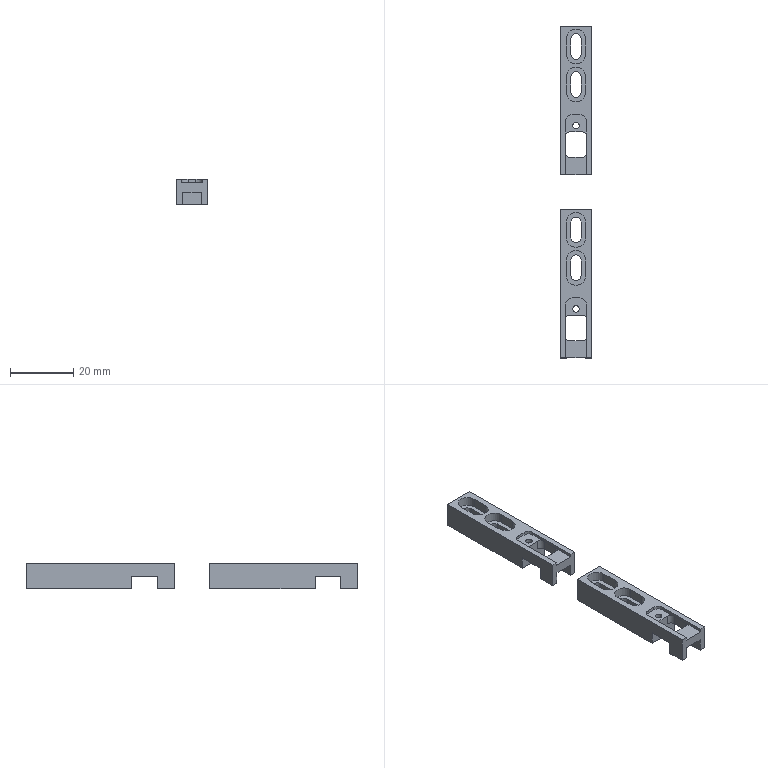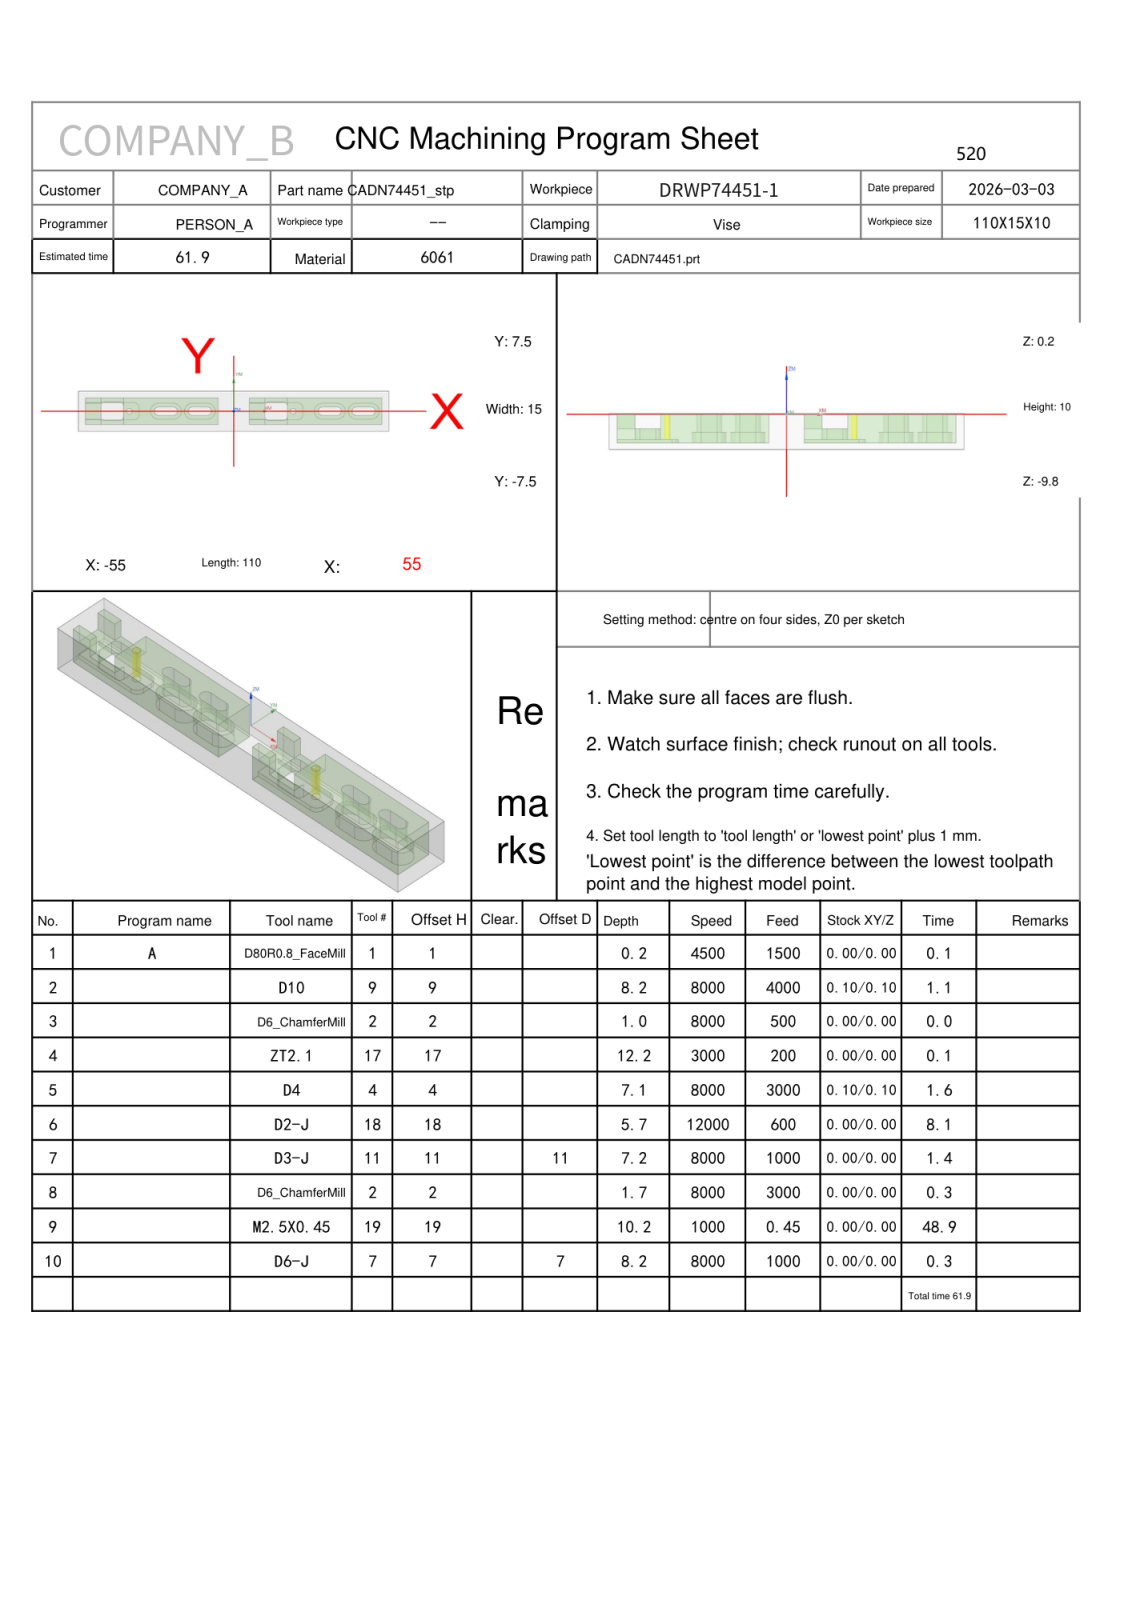NC program | NX | posted by the shop | part box 10 x 105 x 8 mm
Lines 1 to 2024 of 4761:
%
O0001
(Machine time: 108.11 MIN)
(===Total Tool:9===)
(T1=D80R0.8 FaceMill D=80.  R=0.8  D-  H01 Z=0.    )
(T9=D10     D=10.  R=0.   D-  H09 Z=-8.   )
(T2=D6_ChamferMill   D=6.   R=0.   D-  H02 Z=-1.5  )
(T17=ZT2.1  D=2.1  DR_a=118 D-  H17 Z=-12.  )
(T4=D4      D=4.   R=0.   D-  H04 Z=-6.9  )
(T18=D2-J   D=2.   R=0.   D18 H18 Z=-5.5  )
(T11=D3-J   D=3.   R=0.   D11 H11 Z=-7.   )
(T19=M2.5X0.45 D=2.05 DR_a=180 D-  H19 Z=-10.  )
(T7=D6-J    D=6.   R=0.   D7  H07 Z=-8.   )
G80 G90 G17 G49 G40
G91 G28 Z0
M01
N1 T01 M06
(D80R0.8 FaceMill  D=80. R=0.8 H=01 ce=0.00 di=0.00)
G00 G90 G54 X-97.5 Y0.0 M03 S4500
G43 H01 Z50.
M08
Z2.
G01 Z0.0 F1500.
X-92.5
X92.5
X97.5
Z2.
G00 Z50.
G91 G28 Z0.0
M05
M09
G91 G28 Z0.0
M01
N2 T09 M06
(D10  D=10. R=0. H=09 ce=0.10 di=0.10)
G00 G90 G54 X57.481 Y6.032 M03 S8000
G43 H09 Z50.
M08
Z1.
G01 X57.6 Y5.554 Z.974 F4000.
Y-5.554 Z.392
X57.266 Y-6.898 Z.319
X56.584 Y-8.104 Z.247
X55.604 Y-9.084 Z.174
X54.398 Y-9.766 Z.102
X53.054 Y-10.1 Z.029
X52.5 Z0.0
X5.5 Z-.184
G02 X.4 Y-5. Z-.215 I0.0 J5.1
G01 Y5. Z-.254
G02 X5.5 Y10.1 Z-.286 I5.1 J0.0
G01 X52.5 Z-.47
G02 X57.6 Y5. Z-.501 I0.0 J-5.1
G01 Y-5. Z-.54
G02 X52.5 Y-10.1 Z-.571 I-5.1 J0.0
G01 X5.5 Z-.755
G02 X.4 Y-5. Z-.787 I0.0 J5.1
G01 Y5. Z-.826
G02 X5.5 Y10.1 Z-.857 I5.1 J0.0
G01 X52.5 Z-1.041
G02 X57.6 Y5. Z-1.072 I0.0 J-5.1
G01 Y-5. Z-1.112
G02 X52.5 Y-10.1 Z-1.143 I-5.1 J0.0
G01 X5.5 Z-1.327
G02 X.4 Y-5. Z-1.358 I0.0 J5.1
G01 Y5. Z-1.397
G02 X5.5 Y10.1 Z-1.429 I5.1 J0.0
G01 X52.5 Z-1.612
G02 X57.6 Y5. Z-1.644 I0.0 J-5.1
G01 Y-5. Z-1.683
G02 X52.5 Y-10.1 Z-1.714 I-5.1 J0.0
G01 X5.5 Z-1.898
G02 X.4 Y-5. Z-1.93 I0.0 J5.1
G01 Y5. Z-1.969
G02 X5.5 Y10.1 Z-2. I5.1 J0.0
G01 X52.5 Z-2.184
G02 X57.6 Y5. Z-2.215 I0.0 J-5.1
G01 Y-5. Z-2.254
G02 X52.5 Y-10.1 Z-2.286 I-5.1 J0.0
G01 X5.5 Z-2.47
G02 X.4 Y-5. Z-2.501 I0.0 J5.1
G01 Y5. Z-2.54
G02 X5.5 Y10.1 Z-2.571 I5.1 J0.0
G01 X52.5 Z-2.755
G02 X57.6 Y5. Z-2.787 I0.0 J-5.1
G01 Y-5. Z-2.826
G02 X52.5 Y-10.1 Z-2.857 I-5.1 J0.0
G01 X5.5 Z-3.041
G02 X.4 Y-5. Z-3.072 I0.0 J5.1
G01 Y5. Z-3.112
G02 X5.5 Y10.1 Z-3.143 I5.1 J0.0
G01 X52.5 Z-3.327
G02 X57.6 Y5. Z-3.358 I0.0 J-5.1
G01 Y-5. Z-3.397
G02 X52.5 Y-10.1 Z-3.429 I-5.1 J0.0
G01 X5.5 Z-3.612
G02 X.4 Y-5. Z-3.644 I0.0 J5.1
G01 Y5. Z-3.683
G02 X5.5 Y10.1 Z-3.714 I5.1 J0.0
G01 X52.5 Z-3.898
G02 X57.6 Y5. Z-3.93 I0.0 J-5.1
G01 Y-5. Z-3.969
G02 X52.5 Y-10.1 Z-4. I-5.1 J0.0
G01 X5.5 Z-4.184
G02 X.4 Y-5. Z-4.215 I0.0 J5.1
G01 Y5. Z-4.254
G02 X5.5 Y10.1 Z-4.286 I5.1 J0.0
G01 X52.5 Z-4.47
G02 X57.6 Y5. Z-4.501 I0.0 J-5.1
G01 Y-5. Z-4.54
G02 X52.5 Y-10.1 Z-4.571 I-5.1 J0.0
G01 X5.5 Z-4.755
G02 X.4 Y-5. Z-4.787 I0.0 J5.1
G01 Y5. Z-4.826
G02 X5.5 Y10.1 Z-4.857 I5.1 J0.0
G01 X52.5 Z-5.041
G02 X57.6 Y5. Z-5.072 I0.0 J-5.1
G01 Y-5. Z-5.112
G02 X52.5 Y-10.1 Z-5.143 I-5.1 J0.0
G01 X5.5 Z-5.327
G02 X.4 Y-5. Z-5.358 I0.0 J5.1
G01 Y5. Z-5.397
G02 X5.5 Y10.1 Z-5.429 I5.1 J0.0
G01 X52.5 Z-5.612
G02 X57.6 Y5. Z-5.644 I0.0 J-5.1
G01 Y-5. Z-5.683
G02 X52.5 Y-10.1 Z-5.714 I-5.1 J0.0
G01 X5.5 Z-5.898
G02 X.4 Y-5. Z-5.93 I0.0 J5.1
G01 Y5. Z-5.969
G02 X5.5 Y10.1 Z-6. I5.1 J0.0
G01 X52.5 Z-6.184
G02 X57.6 Y5. Z-6.215 I0.0 J-5.1
G01 Y-5. Z-6.254
G02 X52.5 Y-10.1 Z-6.286 I-5.1 J0.0
G01 X5.5 Z-6.47
G02 X.4 Y-5. Z-6.501 I0.0 J5.1
G01 Y5. Z-6.54
G02 X5.5 Y10.1 Z-6.571 I5.1 J0.0
G01 X52.5 Z-6.755
G02 X57.6 Y5. Z-6.787 I0.0 J-5.1
G01 Y-5. Z-6.826
G02 X52.5 Y-10.1 Z-6.857 I-5.1 J0.0
G01 X5.5 Z-7.041
G02 X.4 Y-5. Z-7.072 I0.0 J5.1
G01 Y5. Z-7.112
G02 X5.5 Y10.1 Z-7.143 I5.1 J0.0
G01 X52.5 Z-7.327
G02 X57.6 Y5. Z-7.358 I0.0 J-5.1
G01 Y-5. Z-7.397
G02 X52.5 Y-10.1 Z-7.429 I-5.1 J0.0
G01 X5.5 Z-7.612
G02 X.4 Y-5. Z-7.644 I0.0 J5.1
G01 Y5. Z-7.683
G02 X5.5 Y10.1 Z-7.714 I5.1 J0.0
G01 X52.5 Z-7.898
G02 X57.6 Y5. Z-7.93 I0.0 J-5.1
G01 Y-5. Z-7.969
G02 X52.5 Y-10.1 Z-8. I-5.1 J0.0
G01 X5.5
G02 X.4 Y-5. I0.0 J5.1
G01 Y5.
G02 X5.5 Y10.1 I5.1 J0.0
G01 X52.5
G02 X57.6 Y5. I0.0 J-5.1
G01 Y-5.
G02 X52.5 Y-10.1 I-5.1 J0.0
G01 X52.1
Z-7.
G00 Z50.
X-48.081 Y10.1
Z1.
G01 X-29. Z0.0
X-5.5 Z-.092
G02 X-.4 Y5. Z-.123 I0.0 J-5.1
G01 Y-5. Z-.162
G02 X-5.5 Y-10.1 Z-.194 I-5.1 J0.0
G01 X-52.5 Z-.378
G02 X-57.6 Y-5. Z-.409 I0.0 J5.1
G01 Y5. Z-.448
G02 X-52.5 Y10.1 Z-.479 I5.1 J0.0
G01 X-5.5 Z-.663
G02 X-.4 Y5. Z-.695 I0.0 J-5.1
G01 Y-5. Z-.734
G02 X-5.5 Y-10.1 Z-.765 I-5.1 J0.0
G01 X-52.5 Z-.949
G02 X-57.6 Y-5. Z-.98 I0.0 J5.1
G01 Y5. Z-1.02
G02 X-52.5 Y10.1 Z-1.051 I5.1 J0.0
G01 X-5.5 Z-1.235
G02 X-.4 Y5. Z-1.266 I0.0 J-5.1
G01 Y-5. Z-1.305
G02 X-5.5 Y-10.1 Z-1.337 I-5.1 J0.0
G01 X-52.5 Z-1.521
G02 X-57.6 Y-5. Z-1.552 I0.0 J5.1
G01 Y5. Z-1.591
G02 X-52.5 Y10.1 Z-1.622 I5.1 J0.0
G01 X-5.5 Z-1.806
G02 X-.4 Y5. Z-1.838 I0.0 J-5.1
G01 Y-5. Z-1.877
G02 X-5.5 Y-10.1 Z-1.908 I-5.1 J0.0
G01 X-52.5 Z-2.092
G02 X-57.6 Y-5. Z-2.123 I0.0 J5.1
G01 Y5. Z-2.162
G02 X-52.5 Y10.1 Z-2.194 I5.1 J0.0
G01 X-5.5 Z-2.378
G02 X-.4 Y5. Z-2.409 I0.0 J-5.1
G01 Y-5. Z-2.448
G02 X-5.5 Y-10.1 Z-2.479 I-5.1 J0.0
G01 X-52.5 Z-2.663
G02 X-57.6 Y-5. Z-2.695 I0.0 J5.1
G01 Y5. Z-2.734
G02 X-52.5 Y10.1 Z-2.765 I5.1 J0.0
G01 X-5.5 Z-2.949
G02 X-.4 Y5. Z-2.98 I0.0 J-5.1
G01 Y-5. Z-3.02
G02 X-5.5 Y-10.1 Z-3.051 I-5.1 J0.0
G01 X-52.5 Z-3.235
G02 X-57.6 Y-5. Z-3.266 I0.0 J5.1
G01 Y5. Z-3.305
G02 X-52.5 Y10.1 Z-3.337 I5.1 J0.0
G01 X-5.5 Z-3.521
G02 X-.4 Y5. Z-3.552 I0.0 J-5.1
G01 Y-5. Z-3.591
G02 X-5.5 Y-10.1 Z-3.622 I-5.1 J0.0
G01 X-52.5 Z-3.806
G02 X-57.6 Y-5. Z-3.838 I0.0 J5.1
G01 Y5. Z-3.877
G02 X-52.5 Y10.1 Z-3.908 I5.1 J0.0
G01 X-5.5 Z-4.092
G02 X-.4 Y5. Z-4.123 I0.0 J-5.1
G01 Y-5. Z-4.162
G02 X-5.5 Y-10.1 Z-4.194 I-5.1 J0.0
G01 X-52.5 Z-4.378
G02 X-57.6 Y-5. Z-4.409 I0.0 J5.1
G01 Y5. Z-4.448
G02 X-52.5 Y10.1 Z-4.479 I5.1 J0.0
G01 X-5.5 Z-4.663
G02 X-.4 Y5. Z-4.695 I0.0 J-5.1
G01 Y-5. Z-4.734
G02 X-5.5 Y-10.1 Z-4.765 I-5.1 J0.0
G01 X-52.5 Z-4.949
G02 X-57.6 Y-5. Z-4.98 I0.0 J5.1
G01 Y5. Z-5.02
G02 X-52.5 Y10.1 Z-5.051 I5.1 J0.0
G01 X-5.5 Z-5.235
G02 X-.4 Y5. Z-5.266 I0.0 J-5.1
G01 Y-5. Z-5.305
G02 X-5.5 Y-10.1 Z-5.337 I-5.1 J0.0
G01 X-52.5 Z-5.521
G02 X-57.6 Y-5. Z-5.552 I0.0 J5.1
G01 Y5. Z-5.591
G02 X-52.5 Y10.1 Z-5.622 I5.1 J0.0
G01 X-5.5 Z-5.806
G02 X-.4 Y5. Z-5.838 I0.0 J-5.1
G01 Y-5. Z-5.877
G02 X-5.5 Y-10.1 Z-5.908 I-5.1 J0.0
G01 X-52.5 Z-6.092
G02 X-57.6 Y-5. Z-6.123 I0.0 J5.1
G01 Y5. Z-6.162
G02 X-52.5 Y10.1 Z-6.194 I5.1 J0.0
G01 X-5.5 Z-6.378
G02 X-.4 Y5. Z-6.409 I0.0 J-5.1
G01 Y-5. Z-6.448
G02 X-5.5 Y-10.1 Z-6.479 I-5.1 J0.0
G01 X-52.5 Z-6.663
G02 X-57.6 Y-5. Z-6.695 I0.0 J5.1
G01 Y5. Z-6.734
G02 X-52.5 Y10.1 Z-6.765 I5.1 J0.0
G01 X-5.5 Z-6.949
G02 X-.4 Y5. Z-6.98 I0.0 J-5.1
G01 Y-5. Z-7.02
G02 X-5.5 Y-10.1 Z-7.051 I-5.1 J0.0
G01 X-52.5 Z-7.235
G02 X-57.6 Y-5. Z-7.266 I0.0 J5.1
G01 Y5. Z-7.305
G02 X-52.5 Y10.1 Z-7.337 I5.1 J0.0
G01 X-5.5 Z-7.521
G02 X-.4 Y5. Z-7.552 I0.0 J-5.1
G01 Y-5. Z-7.591
G02 X-5.5 Y-10.1 Z-7.622 I-5.1 J0.0
G01 X-52.5 Z-7.806
G02 X-57.6 Y-5. Z-7.838 I0.0 J5.1
G01 Y5. Z-7.877
G02 X-52.5 Y10.1 Z-7.908 I5.1 J0.0
G01 X-29. Z-8.
X-5.5
G02 X-.4 Y5. I0.0 J-5.1
G01 Y-5.
G02 X-5.5 Y-10.1 I-5.1 J0.0
G01 X-52.5
G02 X-57.6 Y-5. I0.0 J5.1
G01 Y5.
G02 X-52.5 Y10.1 I5.1 J0.0
G01 X-29.
X-28.6
Z-7.
G00 Z50.
G91 G28 Z0.0
M05
M09
G91 G28 Z0.0
M01
N3 T02 M06
(D6_ChamferMill  D=6. R=0. H=02 ce=0.00 di=0.10)
G00 G90 G54 X21. Y0.0 M03 S8000
G43 H02 Z50.
M08
G98 G81 X21. Y0.0 Z-.8 R1. F500.
X-37.
G80
G00 Z50.
G91 G28 Z0.0
M05
M09
G91 G28 Z0.0
M01
N4 T17 M06
(ZT2.1 D=2.1 DR_a=118 H=17)
G00 G90 G54 X21. Y0.0 M03 S3000
G43 H17 Z50.
M08
G98 G83 X21. Y0.0 Z-12. R1. F200. Q2.
X-37.
G80
G00 Z50.
G91 G28 Z0.0
M05
M09
G91 G28 Z0.0
M01
N5 T04 M06
(D4  D=4. R=0. H=04 ce=0.10 di=0.10)
G00 G90 G54 X13.819 Y-1.4 M03 S8000
G43 H04 Z50.
M08
Z1.
G01 X16.9 Z.839 F2000.
Y1.4 Z.692
X13.1 Z.493
Y-1.4 Z.346
X16.9 Z.147
Y1.4 Z0.0
X13.1 Z-.083
Y-1.4 Z-.144
X16.9 Z-.227
Y1.4 Z-.288
X13.1 Z-.37
Y-1.4 Z-.431
X16.9 Z-.514
Y1.4 Z-.575
X13.1 Z-.658
Y-1.4 Z-.719
X16.9 Z-.802
Y1.4 Z-.863
X13.1 Z-.945
Y-1.4 Z-1.006
X16.9 Z-1.089
Y1.4 Z-1.15
X13.1 Z-1.233
Y-1.4 Z-1.294
X16.9 Z-1.377
Y1.4 Z-1.438
X13.1 Z-1.52
Y-1.4 Z-1.581
X16.9 Z-1.664
Y1.4 Z-1.725
X13.1 Z-1.808
Y-1.4 Z-1.869
X16.9 Z-1.952
Y1.4 Z-2.013
X13.1 Z-2.095
Y-1.4 Z-2.156
X16.9 Z-2.239
Y1.4 Z-2.3
X13.1 Z-2.383
Y-1.4 Z-2.444
X16.9 Z-2.527
Y1.4 Z-2.588
X13.1 Z-2.67
Y-1.4 Z-2.731
X16.9 Z-2.814
Y1.4 Z-2.875
X13.1 Z-2.958
Y-1.4 Z-3.019
X16.9 Z-3.102
Y1.4 Z-3.163
X13.1 Z-3.245
Y-1.4 Z-3.306
X16.9 Z-3.389
Y1.4 Z-3.45
X13.1 Z-3.533
Y-1.4 Z-3.594
X16.9 Z-3.677
Y1.4 Z-3.738
X13.1 Z-3.82
Y-1.4 Z-3.881
X16.9 Z-3.964
Y1.4 Z-4.025
X13.1 Z-4.108
Y-1.4 Z-4.169
X16.9 Z-4.252
Y1.4 Z-4.313
X13.1 Z-4.395
Y-1.4 Z-4.456
X16.9 Z-4.539
Y1.4 Z-4.6
X13.1 Z-4.683
Y-1.4 Z-4.744
X16.9 Z-4.827
Y1.4 Z-4.888
X13.1 Z-4.97
Y-1.4 Z-5.031
X16.9 Z-5.114
Y1.4 Z-5.175
X13.1 Z-5.258
Y-1.4 Z-5.319
X16.9 Z-5.402
Y1.4 Z-5.463
X13.1 Z-5.545
Y-1.4 Z-5.606
X16.9 Z-5.689
Y1.4 Z-5.75
X13.1 Z-5.833
Y-1.4 Z-5.894
X16.9 Z-5.977
Y1.4 Z-6.038
X13.1 Z-6.12
Y-1.4 Z-6.181
X16.9 Z-6.264
Y1.4 Z-6.325
X13.1 Z-6.408
Y-1.4 Z-6.469
X16.9 Z-6.552
Y1.4 Z-6.613
X13.1 Z-6.695
Y-1.4 Z-6.756
X16.9 Z-6.839
Y1.4 Z-6.9
X13.1
Y-1.4
X16.9
Y1.4
X16.5
Z-5.9
G00 Z50.
X-44.181 Y-1.4
Z1.
G01 X-41.1 Z.839
Y1.4 Z.692
X-44.9 Z.493
Y-1.4 Z.346
X-41.1 Z.147
Y1.4 Z0.0
X-44.9 Z-.083
Y-1.4 Z-.144
X-41.1 Z-.227
Y1.4 Z-.288
X-44.9 Z-.37
Y-1.4 Z-.431
X-41.1 Z-.514
Y1.4 Z-.575
X-44.9 Z-.658
Y-1.4 Z-.719
X-41.1 Z-.802
Y1.4 Z-.863
X-44.9 Z-.945
Y-1.4 Z-1.006
X-41.1 Z-1.089
Y1.4 Z-1.15
X-44.9 Z-1.233
Y-1.4 Z-1.294
X-41.1 Z-1.377
Y1.4 Z-1.438
X-44.9 Z-1.52
Y-1.4 Z-1.581
X-41.1 Z-1.664
Y1.4 Z-1.725
X-44.9 Z-1.808
Y-1.4 Z-1.869
X-41.1 Z-1.952
Y1.4 Z-2.013
X-44.9 Z-2.095
Y-1.4 Z-2.156
X-41.1 Z-2.239
Y1.4 Z-2.3
X-44.9 Z-2.383
Y-1.4 Z-2.444
X-41.1 Z-2.527
Y1.4 Z-2.588
X-44.9 Z-2.67
Y-1.4 Z-2.731
X-41.1 Z-2.814
Y1.4 Z-2.875
X-44.9 Z-2.958
Y-1.4 Z-3.019
X-41.1 Z-3.102
Y1.4 Z-3.163
X-44.9 Z-3.245
Y-1.4 Z-3.306
X-41.1 Z-3.389
Y1.4 Z-3.45
X-44.9 Z-3.533
Y-1.4 Z-3.594
X-41.1 Z-3.677
Y1.4 Z-3.738
X-44.9 Z-3.82
Y-1.4 Z-3.881
X-41.1 Z-3.964
Y1.4 Z-4.025
X-44.9 Z-4.108
Y-1.4 Z-4.169
X-41.1 Z-4.252
Y1.4 Z-4.313
X-44.9 Z-4.395
Y-1.4 Z-4.456
X-41.1 Z-4.539
Y1.4 Z-4.6
X-44.9 Z-4.683
Y-1.4 Z-4.744
X-41.1 Z-4.827
Y1.4 Z-4.888
X-44.9 Z-4.97
Y-1.4 Z-5.031
X-41.1 Z-5.114
Y1.4 Z-5.175
X-44.9 Z-5.258
Y-1.4 Z-5.319
X-41.1 Z-5.402
Y1.4 Z-5.463
X-44.9 Z-5.545
Y-1.4 Z-5.606
X-41.1 Z-5.689
Y1.4 Z-5.75
X-44.9 Z-5.833
Y-1.4 Z-5.894
X-41.1 Z-5.977
Y1.4 Z-6.038
X-44.9 Z-6.12
Y-1.4 Z-6.181
X-41.1 Z-6.264
Y1.4 Z-6.325
X-44.9 Z-6.408
Y-1.4 Z-6.469
X-41.1 Z-6.552
Y1.4 Z-6.613
X-44.9 Z-6.695
Y-1.4 Z-6.756
X-41.1 Z-6.839
Y1.4 Z-6.9
X-44.9
Y-1.4
X-41.1
Y1.4
X-41.5
Z-5.9
G00 Z50.
G00 G90 X-43. Y10.1 M03 S8000
Z50.
Z.305
G01 Z-.195 F3000.
Y5.4
X-44.9
Y3.1
X-41.1
Y5.4
X-43.
X-43.5
Z.305
G00 Z.5
X-43. Y10.1
Z.11
G01 Z-.39
Y5.4
X-44.9
Y3.1
X-41.1
Y5.4
X-43.
X-43.5
Z.11
G00 Z.305
X-43. Y10.1
Z-.085
G01 Z-.585
Y5.4
X-44.9
Y3.1
X-41.1
Y5.4
X-43.
X-43.5
Z-.085
G00 Z.11
X-43. Y10.1
Z-.28
G01 Z-.78
Y5.4
X-44.9
Y3.1
X-41.1
Y5.4
X-43.
X-43.5
Z-.28
G00 Z-.085
X-43. Y10.1
Z-.475
G01 Z-.975
Y5.4
X-44.9
Y3.1
X-41.1
Y5.4
X-43.
X-43.5
Z-.475
G00 Z-.28
X-43. Y10.1
Z-.67
G01 Z-1.17
Y5.4
X-44.9
Y3.1
X-41.1
Y5.4
X-43.
X-43.5
Z-.67
G00 Z-.475
X-43. Y10.1
Z-.865
G01 Z-1.365
Y5.4
X-44.9
Y3.1
X-41.1
Y5.4
X-43.
X-43.5
Z-.865
G00 Z-.67
X-43. Y10.1
Z-1.06
G01 Z-1.56
Y5.4
X-44.9
Y3.1
X-41.1
Y5.4
X-43.
X-43.5
Z-1.06
G00 Z-.865
X-43. Y10.1
Z-1.255
G01 Z-1.755
Y5.4
X-44.9
Y3.1
X-41.1
Y5.4
X-43.
X-43.5
Z-1.255
G00 Z-1.06
X-43. Y10.1
Z-1.45
G01 Z-1.95
Y5.4
X-44.9
Y3.1
X-41.1
Y5.4
X-43.
X-43.5
Z-1.45
G00 Z-1.255
X-43. Y10.1
Z-1.645
G01 Z-2.145
Y5.4
X-44.9
Y3.1
X-41.1
Y5.4
X-43.
X-43.5
Z-1.645
G00 Z-1.45
X-43. Y10.1
Z-1.84
G01 Z-2.34
Y5.4
X-44.9
Y3.1
X-41.1
Y5.4
X-43.
X-43.5
Z-1.84
G00 Z-1.645
X-43. Y10.1
Z-2.035
G01 Z-2.535
Y5.4
X-44.9
Y3.1
X-41.1
Y5.4
X-43.
X-43.5
Z-2.035
G00 Z-1.84
X-43. Y10.1
Z-2.23
G01 Z-2.73
Y5.4
X-44.9
Y3.1
X-41.1
Y5.4
X-43.
X-43.5
Z-2.23
G00 Z-2.035
X-43. Y10.1
Z-2.425
G01 Z-2.925
Y5.4
X-44.9
Y3.1
X-41.1
Y5.4
X-43.
X-43.5
Z-2.425
G00 Z-2.23
X-43. Y10.1
Z-2.62
G01 Z-3.12
Y5.4
X-44.9
Y3.1
X-41.1
Y5.4
X-43.
X-43.5
Z-2.62
G00 Z-2.425
X-43. Y10.1
Z-2.815
G01 Z-3.315
Y5.4
X-44.9
Y3.1
X-41.1
Y5.4
X-43.
X-43.5
Z-2.815
G00 Z-2.62
X-43. Y10.1
Z-3.01
G01 Z-3.51
Y5.4
X-44.9
Y3.1
X-41.1
Y5.4
X-43.
X-43.5
Z-3.01
G00 Z-2.815
X-43. Y10.1
Z-3.205
G01 Z-3.705
Y5.4
X-44.9
Y3.1
X-41.1
Y5.4
X-43.
X-43.5
Z-3.205
G00 Z-3.01
X-43. Y10.1
Z-3.4
G01 Z-3.9
Y5.4
X-44.9
Y3.1
X-41.1
Y5.4
X-43.
X-43.5
Z-3.4
G00 Z50.
X-57.6 Y0.0
Z.305
G01 Z-.195
X-52.9
Y-.9
X-45.6
Y.9
X-52.9
Y0.0
Y-.5
Z.305
G00 Z50.
X-57.6 Y0.0
Z.11
G01 Z-.39
X-52.9
Y-.9
X-45.6
Y.9
X-52.9
Y0.0
Y-.5
Z.11
G00 Z.305
X-57.6 Y0.0
Z-.085
G01 Z-.585
X-52.9
Y-.9
X-45.6
Y.9
X-52.9
Y0.0
Y-.5
Z-.085
G00 Z.11
X-57.6 Y0.0
Z-.28
G01 Z-.78
X-52.9
Y-.9
X-45.6
Y.9
X-52.9
Y0.0
Y-.5
Z-.28
G00 Z-.085
X-57.6 Y0.0
Z-.475
G01 Z-.975
X-52.9
Y-.9
X-45.6
Y.9
X-52.9
Y0.0
Y-.5
Z-.475
G00 Z-.28
X-57.6 Y0.0
Z-.67
G01 Z-1.17
X-52.9
Y-.9
X-45.6
Y.9
X-52.9
Y0.0
Y-.5
Z-.67
G00 Z-.475
X-57.6 Y0.0
Z-.865
G01 Z-1.365
X-52.9
Y-.9
X-45.6
Y.9
X-52.9
Y0.0
Y-.5
Z-.865
G00 Z-.67
X-57.6 Y0.0
Z-1.06
G01 Z-1.56
X-52.9
Y-.9
X-45.6
Y.9
X-52.9
Y0.0
Y-.5
Z-1.06
G00 Z-.865
X-57.6 Y0.0
Z-1.255
G01 Z-1.755
X-52.9
Y-.9
X-45.6
Y.9
X-52.9
Y0.0
Y-.5
Z-1.255
G00 Z-1.06
X-57.6 Y0.0
Z-1.45
G01 Z-1.95
X-52.9
Y-.9
X-45.6
Y.9
X-52.9
Y0.0
Y-.5
Z-1.45
G00 Z-1.255
X-57.6 Y0.0
Z-1.645
G01 Z-2.145
X-52.9
Y-.9
X-45.6
Y.9
X-52.9
Y0.0
Y-.5
Z-1.645
G00 Z-1.45
X-57.6 Y0.0
Z-1.84
G01 Z-2.34
X-52.9
Y-.9
X-45.6
Y.9
X-52.9
Y0.0
Y-.5
Z-1.84
G00 Z-1.645
X-57.6 Y0.0
Z-2.035
G01 Z-2.535
X-52.9
Y-.9
X-45.6
Y.9
X-52.9
Y0.0
Y-.5
Z-2.035
G00 Z-1.84
X-57.6 Y0.0
Z-2.23
G01 Z-2.73
X-52.9
Y-.9
X-45.6
Y.9
X-52.9
Y0.0
Y-.5
Z-2.23
G00 Z-2.035
X-57.6 Y0.0
Z-2.425
G01 Z-2.925
X-52.9
Y-.9
X-45.6
Y.9
X-52.9
Y0.0
Y-.5
Z-2.425
G00 Z-2.23
X-57.6 Y0.0
Z-2.62
G01 Z-3.12
X-52.9
Y-.9
X-45.6
Y.9
X-52.9
Y0.0
Y-.5
Z-2.62
G00 Z-2.425
X-57.6 Y0.0
Z-2.815
G01 Z-3.315
X-52.9
Y-.9
X-45.6
Y.9
X-52.9
Y0.0
Y-.5
Z-2.815
G00 Z-2.62
X-57.6 Y0.0
Z-3.01
G01 Z-3.51
X-52.9
Y-.9
X-45.6
Y.9
X-52.9
Y0.0
Y-.5
Z-3.01
G00 Z-2.815
X-57.6 Y0.0
Z-3.205
G01 Z-3.705
X-52.9
Y-.9
X-45.6
Y.9
X-52.9
Y0.0
Y-.5
Z-3.205
G00 Z-3.01
X-57.6 Y0.0
Z-3.4
G01 Z-3.9
X-52.9
Y-.9
X-45.6
Y.9
X-52.9
Y0.0
Y-.5
Z-3.4
G00 Z50.
X-43. Y-10.1
Z.305
G01 Z-.195
Y-5.4
X-41.1
Y-3.1
X-44.9
Y-5.4
X-43.
X-42.5
Z.305
G00 Z.5
X-43. Y-10.1
Z.11
G01 Z-.39
Y-5.4
X-41.1
Y-3.1
X-44.9
Y-5.4
X-43.
X-42.5
Z.11
G00 Z.305
X-43. Y-10.1
Z-.085
G01 Z-.585
Y-5.4
X-41.1
Y-3.1
X-44.9
Y-5.4
X-43.
X-42.5
Z-.085
G00 Z.11
X-43. Y-10.1
Z-.28
G01 Z-.78
Y-5.4
X-41.1
Y-3.1
X-44.9
Y-5.4
X-43.
X-42.5
Z-.28
G00 Z-.085
X-43. Y-10.1
Z-.475
G01 Z-.975
Y-5.4
X-41.1
Y-3.1
X-44.9
Y-5.4
X-43.
X-42.5
Z-.475
G00 Z-.28
X-43. Y-10.1
Z-.67
G01 Z-1.17
Y-5.4
X-41.1
Y-3.1
X-44.9
Y-5.4
X-43.
X-42.5
Z-.67
G00 Z-.475
X-43. Y-10.1
Z-.865
G01 Z-1.365
Y-5.4
X-41.1
Y-3.1
X-44.9
Y-5.4
X-43.
X-42.5
Z-.865
G00 Z-.67
X-43. Y-10.1
Z-1.06
G01 Z-1.56
Y-5.4
X-41.1
Y-3.1
X-44.9
Y-5.4
X-43.
X-42.5
Z-1.06
G00 Z-.865
X-43. Y-10.1
Z-1.255
G01 Z-1.755
Y-5.4
X-41.1
Y-3.1
X-44.9
Y-5.4
X-43.
X-42.5
Z-1.255
G00 Z-1.06
X-43. Y-10.1
Z-1.45
G01 Z-1.95
Y-5.4
X-41.1
Y-3.1
X-44.9
Y-5.4
X-43.
X-42.5
Z-1.45
G00 Z-1.255
X-43. Y-10.1
Z-1.645
G01 Z-2.145
Y-5.4
X-41.1
Y-3.1
X-44.9
Y-5.4
X-43.
X-42.5
Z-1.645
G00 Z-1.45
X-43. Y-10.1
Z-1.84
G01 Z-2.34
Y-5.4
X-41.1
Y-3.1
X-44.9
Y-5.4
X-43.
X-42.5
Z-1.84
G00 Z-1.645
X-43. Y-10.1
Z-2.035
G01 Z-2.535
Y-5.4
X-41.1
Y-3.1
X-44.9
Y-5.4
X-43.
X-42.5
Z-2.035
G00 Z-1.84
X-43. Y-10.1
Z-2.23
G01 Z-2.73
Y-5.4
X-41.1
Y-3.1
X-44.9
Y-5.4
X-43.
X-42.5
Z-2.23
G00 Z-2.035
X-43. Y-10.1
Z-2.425
G01 Z-2.925
Y-5.4
X-41.1
Y-3.1
X-44.9
Y-5.4
X-43.
X-42.5
Z-2.425
G00 Z-2.23
X-43. Y-10.1
Z-2.62
G01 Z-3.12
Y-5.4
X-41.1
Y-3.1
X-44.9
Y-5.4
X-43.
X-42.5
Z-2.62
G00 Z-2.425
X-43. Y-10.1
Z-2.815
G01 Z-3.315
Y-5.4
X-41.1
Y-3.1
X-44.9
Y-5.4
X-43.
X-42.5
Z-2.815
G00 Z-2.62
X-43. Y-10.1
Z-3.01
G01 Z-3.51
Y-5.4
X-41.1
Y-3.1
X-44.9
Y-5.4
X-43.
X-42.5
Z-3.01
G00 Z-2.815
X-43. Y-10.1
Z-3.205
G01 Z-3.705
Y-5.4
X-41.1
Y-3.1
X-44.9
Y-5.4
X-43.
X-42.5
Z-3.205
G00 Z-3.01
X-43. Y-10.1
Z-3.4
G01 Z-3.9
Y-5.4
X-41.1
Y-3.1
X-44.9
Y-5.4
X-43.
X-42.5
Z-3.4
G00 Z50.
X15. Y10.1
Z.305
G01 Z-.195
Y5.4
X13.1
Y3.1
X16.9
Y5.4
X15.
X14.5
Z.305
G00 Z.5
X15. Y10.1
Z.11
G01 Z-.39
Y5.4
X13.1
Y3.1
X16.9
Y5.4
X15.
X14.5
Z.11
G00 Z.305
X15. Y10.1
Z-.085
G01 Z-.585
Y5.4
X13.1
Y3.1
X16.9
Y5.4
X15.
X14.5
Z-.085
G00 Z.11
X15. Y10.1
Z-.28
G01 Z-.78
Y5.4
X13.1
Y3.1
X16.9
Y5.4
X15.
X14.5
Z-.28
G00 Z-.085
X15. Y10.1
Z-.475
G01 Z-.975
Y5.4
X13.1
Y3.1
X16.9
Y5.4
X15.
X14.5
Z-.475
G00 Z-.28
X15. Y10.1
Z-.67
G01 Z-1.17
Y5.4
X13.1
Y3.1
X16.9
Y5.4
X15.
X14.5
Z-.67
G00 Z-.475
X15. Y10.1
Z-.865
G01 Z-1.365
Y5.4
X13.1
Y3.1
X16.9
Y5.4
X15.
X14.5
Z-.865
G00 Z-.67
X15. Y10.1
Z-1.06
G01 Z-1.56
Y5.4
X13.1
Y3.1
X16.9
Y5.4
X15.
X14.5
Z-1.06
G00 Z-.865
X15. Y10.1
Z-1.255
G01 Z-1.755
Y5.4
X13.1
Y3.1
X16.9
Y5.4
X15.
X14.5
Z-1.255
G00 Z-1.06
X15. Y10.1
Z-1.45
G01 Z-1.95
Y5.4
X13.1
Y3.1
X16.9
Y5.4
X15.
X14.5
Z-1.45
G00 Z-1.255
X15. Y10.1
Z-1.645
G01 Z-2.145
Y5.4
X13.1
Y3.1
X16.9
Y5.4
X15.
X14.5
Z-1.645
G00 Z-1.45
X15. Y10.1
Z-1.84
G01 Z-2.34
Y5.4
X13.1
Y3.1
X16.9
Y5.4
X15.
X14.5
Z-1.84
G00 Z-1.645
X15. Y10.1
Z-2.035
G01 Z-2.535
Y5.4
X13.1
Y3.1
X16.9
Y5.4
X15.
X14.5
Z-2.035
G00 Z-1.84
X15. Y10.1
Z-2.23
G01 Z-2.73
Y5.4
X13.1
Y3.1
X16.9
Y5.4
X15.
X14.5
Z-2.23
G00 Z-2.035
X15. Y10.1
Z-2.425
G01 Z-2.925
Y5.4
X13.1
Y3.1
X16.9
Y5.4
X15.
X14.5
Z-2.425
G00 Z-2.23
X15. Y10.1
Z-2.62
G01 Z-3.12
Y5.4
X13.1
Y3.1
X16.9
Y5.4
X15.
X14.5
Z-2.62
G00 Z-2.425
X15. Y10.1
Z-2.815
G01 Z-3.315
Y5.4
X13.1
Y3.1
X16.9
Y5.4
X15.
X14.5
Z-2.815
G00 Z-2.62
X15. Y10.1
Z-3.01
G01 Z-3.51
Y5.4
X13.1
Y3.1
X16.9
Y5.4
X15.
X14.5
Z-3.01
G00 Z-2.815
X15. Y10.1
Z-3.205
G01 Z-3.705
Y5.4
X13.1
Y3.1
X16.9
Y5.4
X15.
X14.5
Z-3.205
G00 Z-3.01
X15. Y10.1
Z-3.4
G01 Z-3.9
Y5.4
X13.1
Y3.1
X16.9
Y5.4
X15.
X14.5
Z-3.4
G00 Z50.
X13.8 Y10.1
Z.305
G01 Z-.195
Y0.0
X11.4
Y.9
X5.1
Y-.9
X11.4
Y0.0
Y.5
Z.305
G00 Z50.
X13.8 Y10.1
Z.11
G01 Z-.39
Y0.0
X11.4
Y.9
X5.1
Y-.9
X11.4
Y0.0
Y.5
Z.11
G00 Z50.
X13.8 Y10.1
Z-.085
G01 Z-.585
Y0.0
X11.4
Y.9
X5.1
Y-.9
X11.4
Y0.0
Y.5
Z-.085
G00 Z50.
X13.8 Y10.1
Z-.28
G01 Z-.78
Y0.0
X11.4
Y.9
X5.1
Y-.9
X11.4
Y0.0
Y.5
Z-.28
G00 Z50.
X13.8 Y10.1
Z-.475
G01 Z-.975
Y0.0
X11.4
Y.9
X5.1
Y-.9
X11.4
Y0.0
Y.5
Z-.475
G00 Z50.
X13.8 Y10.1
Z-.67
G01 Z-1.17
Y0.0
X11.4
Y.9
X5.1
Y-.9
X11.4
Y0.0
Y.5
Z-.67
G00 Z50.
X13.8 Y10.1
Z-.865
G01 Z-1.365
Y0.0
X11.4
Y.9
X5.1
Y-.9
X11.4
Y0.0
Y.5
Z-.865
G00 Z50.
X13.8 Y10.1
Z-1.06
G01 Z-1.56
Y0.0
X11.4
Y.9
X5.1
Y-.9
X11.4
Y0.0
Y.5
Z-1.06
G00 Z50.
X13.8 Y10.1
Z-1.255
G01 Z-1.755
Y0.0
X11.4
Y.9
X5.1
Y-.9
X11.4
Y0.0
Y.5
Z-1.255
G00 Z50.
X13.8 Y10.1
Z-1.45
G01 Z-1.95
Y0.0
X11.4
Y.9
X5.1
Y-.9
X11.4
Y0.0
Y.5
Z-1.45
G00 Z50.
X13.8 Y10.1
Z-1.645
G01 Z-2.145
Y0.0
X11.4
Y.9
X5.1
Y-.9
X11.4
Y0.0
Y.5
Z-1.645
G00 Z50.
X13.8 Y10.1
Z-1.84
G01 Z-2.34
Y0.0
X11.4
Y.9
X5.1
Y-.9
X11.4
Y0.0
Y.5
Z-1.84
G00 Z50.
X13.8 Y10.1
Z-2.035
G01 Z-2.535
Y0.0
X11.4
Y.9
X5.1
Y-.9
X11.4
Y0.0
Y.5
Z-2.035
G00 Z50.
X13.8 Y10.1
Z-2.23
G01 Z-2.73
Y0.0
X11.4
Y.9
X5.1
Y-.9
X11.4
Y0.0
Y.5
Z-2.23
G00 Z50.
X13.8 Y10.1
Z-2.425
G01 Z-2.925
Y0.0
X11.4
Y.9
X5.1
Y-.9
X11.4
Y0.0
Y.5
Z-2.425
G00 Z50.
X13.8 Y10.1
Z-2.62
G01 Z-3.12
Y0.0
X11.4
Y.9
X5.1
Y-.9
X11.4
Y0.0
Y.5
Z-2.62
G00 Z50.
X13.8 Y10.1
Z-2.815
G01 Z-3.315
Y0.0
X11.4
Y.9
X5.1
Y-.9
X11.4
Y0.0
Y.5
Z-2.815
G00 Z50.
X13.8 Y10.1
Z-3.01
G01 Z-3.51
Y0.0
X11.4
Y.9
X5.1
Y-.9
X11.4
Y0.0
Y.5
Z-3.01
G00 Z50.
X13.8 Y10.1
Z-3.205
G01 Z-3.705
Y0.0
X11.4
Y.9
X5.1
Y-.9
X11.4
Y0.0
Y.5
Z-3.205
G00 Z-3.01
X.4 Y0.0
Z-3.4
G01 Z-3.9
X5.1
Y-.9
X11.4
Y.9
X5.1
Y0.0
Y-.5
Z-3.4
G00 Z50.
X15. Y-10.1
Z.305
G01 Z-.195
Y-5.4
X16.9
Y-3.1
X13.1
Y-5.4
X15.
X15.5
Z.305
G00 Z.5
X15. Y-10.1
Z.11
G01 Z-.39
Y-5.4
X16.9
Y-3.1
X13.1
Y-5.4
X15.
X15.5
Z.11
G00 Z.305
X15. Y-10.1
Z-.085
G01 Z-.585
Y-5.4
X16.9
Y-3.1
X13.1
Y-5.4
X15.
X15.5
Z-.085
G00 Z.11
X15. Y-10.1
Z-.28
G01 Z-.78
Y-5.4
X16.9
Y-3.1
X13.1
Y-5.4
X15.
X15.5
Z-.28
G00 Z-.085
X15. Y-10.1
Z-.475
G01 Z-.975
Y-5.4
X16.9
Y-3.1
X13.1
Y-5.4
X15.
X15.5
Z-.475
G00 Z-.28
X15. Y-10.1
Z-.67
G01 Z-1.17
Y-5.4
X16.9
Y-3.1
X13.1
Y-5.4
X15.
X15.5
Z-.67
G00 Z-.475
X15. Y-10.1
Z-.865
G01 Z-1.365
Y-5.4
X16.9
Y-3.1
X13.1
Y-5.4
X15.
X15.5
Z-.865
G00 Z-.67
X15. Y-10.1
Z-1.06
G01 Z-1.56
Y-5.4
X16.9
Y-3.1
X13.1
Y-5.4
X15.
X15.5
Z-1.06
G00 Z-.865
X15. Y-10.1
Z-1.255
G01 Z-1.755
Y-5.4
X16.9
Y-3.1
X13.1
Y-5.4
X15.
X15.5
Z-1.255
G00 Z-1.06
X15. Y-10.1
Z-1.45
G01 Z-1.95
Y-5.4
X16.9
Y-3.1
X13.1
Y-5.4
X15.
X15.5
Z-1.45
G00 Z-1.255
X15. Y-10.1
Z-1.645
G01 Z-2.145
Y-5.4
X16.9
Y-3.1
X13.1
Y-5.4
X15.
X15.5
Z-1.645
G00 Z-1.45
X15. Y-10.1
Z-1.84
G01 Z-2.34
Y-5.4
X16.9
Y-3.1
X13.1
Y-5.4
X15.
X15.5
Z-1.84
G00 Z-1.645
X15. Y-10.1
Z-2.035
G01 Z-2.535
Y-5.4
X16.9
Y-3.1
X13.1
Y-5.4
X15.
X15.5
Z-2.035
G00 Z-1.84
X15. Y-10.1
Z-2.23
G01 Z-2.73
Y-5.4
X16.9
Y-3.1
X13.1
Y-5.4
X15.
X15.5
Z-2.23
G00 Z-2.035
X15. Y-10.1
Z-2.425
G01 Z-2.925
Y-5.4
X16.9
Y-3.1
X13.1
Y-5.4
X15.
X15.5
Z-2.425
G00 Z-2.23
X15. Y-10.1
Z-2.62
G01 Z-3.12
Y-5.4
X16.9
Y-3.1
X13.1
Y-5.4
X15.
X15.5
Z-2.62
G00 Z-2.425
X15. Y-10.1
Z-2.815
G01 Z-3.315
Y-5.4
X16.9
Y-3.1
X13.1
Y-5.4
X15.
X15.5
Z-2.815
G00 Z-2.62
X15. Y-10.1
Z-3.01
G01 Z-3.51
Y-5.4
X16.9
Y-3.1
X13.1
Y-5.4
X15.
X15.5
Z-3.01
G00 Z-2.815
X15. Y-10.1
Z-3.205
G01 Z-3.705
Y-5.4
X16.9
Y-3.1
X13.1
Y-5.4
X15.
X15.5
Z-3.205
G00 Z-3.01
X15. Y-10.1
Z-3.4
G01 Z-3.9
Y-5.4
X16.9
Y-3.1
X13.1
Y-5.4
X15.
X15.5
Z-3.4
G00 Z50.
G91 G28 Z0.0
M05
M09
G91 G28 Z0.0
M01